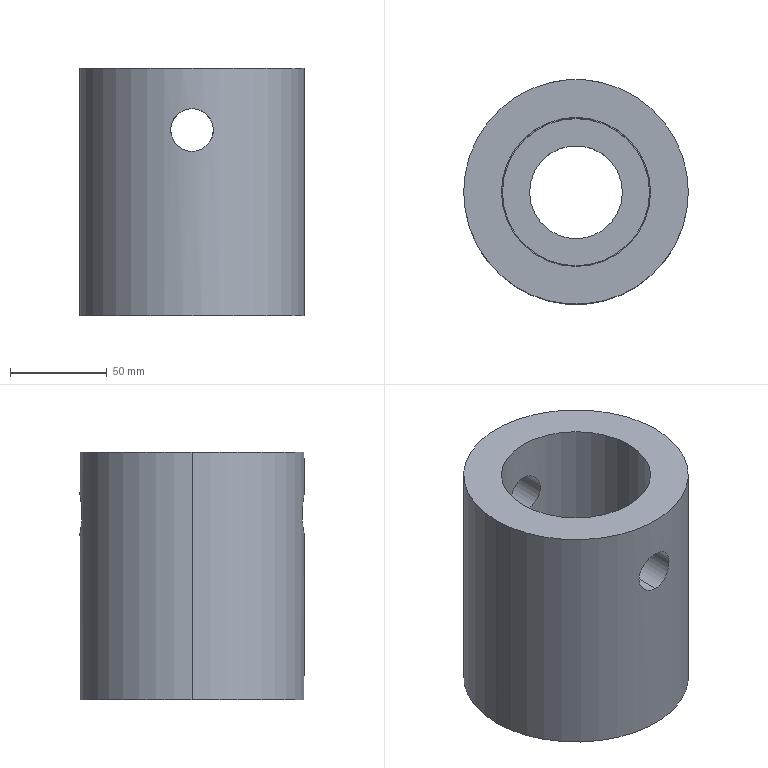Part | SolidWorks | features ICE 4, Extrusion 1 | 1 solid | 19 faces | box 116 x 116 x 128 mm | volume 818395 mm3 | cylinder 14 | plane 5 | commonest cylinder face diameters 22 x4 48 x2 76 x2 77 x2 80 x2 116 x2
STEP:
#1=CARTESIAN_POINT('',(-40.,0.,64.));
#2=VERTEX_POINT('',#1);
#3=CARTESIAN_POINT('',(40.,0.,64.));
#4=VERTEX_POINT('',#3);
#5=CARTESIAN_POINT('',(0.,0.,64.));
#6=DIRECTION('',(0.,0.,1.));
#7=DIRECTION('',(1.,0.,0.));
#8=AXIS2_PLACEMENT_3D('',#5,#6,#7);
#9=CIRCLE('',#8,40.);
#10=EDGE_CURVE('',#2,#4,#9,.T.);
#11=ORIENTED_EDGE('',*,*,#10,.T.);
#12=CARTESIAN_POINT('',(40.,0.,60.));
#13=VERTEX_POINT('',#12);
#14=CARTESIAN_POINT('',(40.,0.,64.));
#15=DIRECTION('',(0.,0.,-1.));
#16=VECTOR('',#15,1000.);
#17=LINE('',#14,#16);
#18=EDGE_CURVE('',#4,#13,#17,.T.);
#19=ORIENTED_EDGE('',*,*,#18,.T.);
#20=CARTESIAN_POINT('',(-40.,0.,60.));
#21=VERTEX_POINT('',#20);
#22=CARTESIAN_POINT('',(0.,0.,60.));
#23=DIRECTION('',(0.,0.,1.));
#24=DIRECTION('',(1.,0.,0.));
#25=AXIS2_PLACEMENT_3D('',#22,#23,#24);
#26=CIRCLE('',#25,40.);
#27=EDGE_CURVE('',#21,#13,#26,.T.);
#28=ORIENTED_EDGE('',*,*,#27,.F.);
#29=CARTESIAN_POINT('',(-40.,0.,64.));
#30=DIRECTION('',(0.,0.,-1.));
#31=VECTOR('',#30,1000.);
#32=LINE('',#29,#31);
#33=EDGE_CURVE('',#2,#21,#32,.T.);
#34=ORIENTED_EDGE('',*,*,#33,.F.);
#35=EDGE_LOOP('',(#11,#19,#28,#34));
#36=FACE_OUTER_BOUND('',#35,.T.);
#37=CARTESIAN_POINT('',(0.,0.,64.));
#38=DIRECTION('',(0.,0.,-1.));
#39=DIRECTION('',(-1.,0.,0.));
#40=AXIS2_PLACEMENT_3D('',#37,#38,#39);
#41=CYLINDRICAL_SURFACE('',#40,40.);
#42=ADVANCED_FACE('',(#36),#41,.F.);
#43=CARTESIAN_POINT('',(0.,-38.5,107.));
#44=VERTEX_POINT('',#43);
#45=CARTESIAN_POINT('',(0.,-38.5,85.));
#46=VERTEX_POINT('',#45);
#47=CARTESIAN_POINT('',(0.,-38.5,107.));
#48=CARTESIAN_POINT('',(0.7309,-38.5,107.));
#49=CARTESIAN_POINT('',(1.449,-38.479,106.928));
#50=CARTESIAN_POINT('',(2.507,-38.42,106.716));
#51=CARTESIAN_POINT('',(2.857,-38.395,106.629));
#52=CARTESIAN_POINT('',(3.55,-38.338,106.418));
#53=CARTESIAN_POINT('',(3.894,-38.304,106.294));
#54=CARTESIAN_POINT('',(4.892,-38.194,105.879));
#55=CARTESIAN_POINT('',(5.522,-38.107,105.541));
#56=CARTESIAN_POINT('',(6.417,-37.963,104.942));
#57=CARTESIAN_POINT('',(6.708,-37.912,104.725));
#58=CARTESIAN_POINT('',(7.264,-37.81,104.268));
#59=CARTESIAN_POINT('',(7.529,-37.758,104.028));
#60=CARTESIAN_POINT('',(8.285,-37.601,103.271));
#61=CARTESIAN_POINT('',(8.739,-37.497,102.719));
#62=CARTESIAN_POINT('',(9.543,-37.301,101.518));
#63=CARTESIAN_POINT('',(9.882,-37.211,100.884));
#64=CARTESIAN_POINT('',(10.294,-37.098,99.893));
#65=CARTESIAN_POINT('',(10.416,-37.064,99.555));
#66=CARTESIAN_POINT('',(10.627,-37.005,98.864));
#67=CARTESIAN_POINT('',(10.716,-36.979,98.509));
#68=CARTESIAN_POINT('',(10.929,-36.917,97.443));
#69=CARTESIAN_POINT('',(11.,-36.895,96.727));
#70=CARTESIAN_POINT('',(11.,-36.895,95.283));
#71=CARTESIAN_POINT('',(10.928,-36.917,94.55));
#72=CARTESIAN_POINT('',(10.645,-36.999,93.136));
#73=CARTESIAN_POINT('',(10.436,-37.06,92.448));
#74=CARTESIAN_POINT('',(10.019,-37.174,91.446));
#75=CARTESIAN_POINT('',(9.863,-37.215,91.117));
#76=CARTESIAN_POINT('',(9.524,-37.304,90.484));
#77=CARTESIAN_POINT('',(9.339,-37.351,90.177));
#78=CARTESIAN_POINT('',(8.942,-37.448,89.584));
#79=CARTESIAN_POINT('',(8.729,-37.498,89.297));
#80=CARTESIAN_POINT('',(8.274,-37.601,88.742));
#81=CARTESIAN_POINT('',(8.03,-37.654,88.474));
#82=CARTESIAN_POINT('',(7.267,-37.811,87.711));
#83=CARTESIAN_POINT('',(6.716,-37.914,87.259));
#84=CARTESIAN_POINT('',(5.527,-38.106,86.463));
#85=CARTESIAN_POINT('',(4.883,-38.195,86.117));
#86=CARTESIAN_POINT('',(3.556,-38.341,85.566));
#87=CARTESIAN_POINT('',(2.87,-38.399,85.356));
#88=CARTESIAN_POINT('',(1.805,-38.459,85.143));
#89=CARTESIAN_POINT('',(1.443,-38.475,85.089));
#90=CARTESIAN_POINT('',(0.7207,-38.495,85.018));
#91=CARTESIAN_POINT('',(0.3602,-38.5,85.));
#92=CARTESIAN_POINT('',(0.,-38.5,85.));
#93=B_SPLINE_CURVE_WITH_KNOTS('',3,(#47,#48,#49,#50,#51,#52,#53,#54,#55,#56,#57,#58,#59,#60,#61,#62,#63,#64,#65,#66,#67,#68,#69,#70,#71,#72,#73,#74,#75,#76,#77,#78,#79,#80,#81,#82,#83,#84,#85,#86,#87,#88,#89,#90,#91,#92),.UNSPECIFIED.,.F.,.F.,(4,2,2,2,2,2,2,2,2,2,2,2,2,2,2,2,2,2,2,2,2,2,4),(0.,0.002161,0.003241,0.004322,0.006482,0.007563,0.008643,0.0108,0.01296,0.01404,0.01513,0.01729,0.01945,0.02161,0.02269,0.02377,0.02485,0.02593,0.02809,0.03025,0.03241,0.03349,0.03457),.UNSPECIFIED.);
#94=EDGE_CURVE('',#44,#46,#93,.T.);
#95=ORIENTED_EDGE('',*,*,#94,.F.);
#96=CARTESIAN_POINT('',(0.,-38.5,85.));
#97=CARTESIAN_POINT('',(-0.3601,-38.5,85.));
#98=CARTESIAN_POINT('',(-0.7197,-38.495,85.018));
#99=CARTESIAN_POINT('',(-1.438,-38.475,85.088));
#100=CARTESIAN_POINT('',(-1.798,-38.46,85.142));
#101=CARTESIAN_POINT('',(-2.87,-38.4,85.356));
#102=CARTESIAN_POINT('',(-3.557,-38.341,85.566));
#103=CARTESIAN_POINT('',(-4.552,-38.231,85.979));
#104=CARTESIAN_POINT('',(-4.877,-38.191,86.133));
#105=CARTESIAN_POINT('',(-5.514,-38.104,86.475));
#106=CARTESIAN_POINT('',(-5.825,-38.058,86.662));
#107=CARTESIAN_POINT('',(-6.718,-37.914,87.26));
#108=CARTESIAN_POINT('',(-7.269,-37.811,87.713));
#109=CARTESIAN_POINT('',(-8.03,-37.654,88.474));
#110=CARTESIAN_POINT('',(-8.274,-37.601,88.743));
#111=CARTESIAN_POINT('',(-8.73,-37.498,89.298));
#112=CARTESIAN_POINT('',(-8.943,-37.448,89.585));
#113=CARTESIAN_POINT('',(-9.538,-37.302,90.474));
#114=CARTESIAN_POINT('',(-9.877,-37.212,91.105));
#115=CARTESIAN_POINT('',(-10.435,-37.06,92.446));
#116=CARTESIAN_POINT('',(-10.645,-37.,93.135));
#117=CARTESIAN_POINT('',(-10.856,-36.938,94.191));
#118=CARTESIAN_POINT('',(-10.91,-36.922,94.548));
#119=CARTESIAN_POINT('',(-10.982,-36.901,95.269));
#120=CARTESIAN_POINT('',(-11.,-36.895,95.636));
#121=CARTESIAN_POINT('',(-11.,-36.895,96.723));
#122=CARTESIAN_POINT('',(-10.929,-36.916,97.44));
#123=CARTESIAN_POINT('',(-10.718,-36.978,98.502));
#124=CARTESIAN_POINT('',(-10.629,-37.004,98.855));
#125=CARTESIAN_POINT('',(-10.418,-37.064,99.55));
#126=CARTESIAN_POINT('',(-10.296,-37.098,99.889));
#127=CARTESIAN_POINT('',(-9.883,-37.211,100.883));
#128=CARTESIAN_POINT('',(-9.545,-37.3,101.515));
#129=CARTESIAN_POINT('',(-8.741,-37.497,102.716));
#130=CARTESIAN_POINT('',(-8.286,-37.601,103.27));
#131=CARTESIAN_POINT('',(-7.53,-37.757,104.027));
#132=CARTESIAN_POINT('',(-7.265,-37.809,104.267));
#133=CARTESIAN_POINT('',(-6.711,-37.912,104.723));
#134=CARTESIAN_POINT('',(-6.419,-37.962,104.94));
#135=CARTESIAN_POINT('',(-5.523,-38.107,105.54));
#136=CARTESIAN_POINT('',(-4.893,-38.194,105.878));
#137=CARTESIAN_POINT('',(-3.568,-38.34,106.43));
#138=CARTESIAN_POINT('',(-2.866,-38.4,106.645));
#139=CARTESIAN_POINT('',(-1.45,-38.479,106.928));
#140=CARTESIAN_POINT('',(-0.7307,-38.5,107.));
#141=CARTESIAN_POINT('',(0.,-38.5,107.));
#142=B_SPLINE_CURVE_WITH_KNOTS('',3,(#96,#97,#98,#99,#100,#101,#102,#103,#104,#105,#106,#107,#108,#109,#110,#111,#112,#113,#114,#115,#116,#117,#118,#119,#120,#121,#122,#123,#124,#125,#126,#127,#128,#129,#130,#131,#132,#133,#134,#135,#136,#137,#138,#139,#140,#141),.UNSPECIFIED.,.F.,.F.,(4,2,2,2,2,2,2,2,2,2,2,2,2,2,2,2,2,2,2,2,2,2,4),(0.03457,0.03565,0.03673,0.03889,0.03997,0.04105,0.04321,0.04429,0.04537,0.04753,0.04969,0.05077,0.05185,0.05401,0.05509,0.05617,0.05833,0.06049,0.06157,0.06265,0.06481,0.06697,0.06913),.UNSPECIFIED.);
#143=EDGE_CURVE('',#46,#44,#142,.T.);
#144=ORIENTED_EDGE('',*,*,#143,.F.);
#145=EDGE_LOOP('',(#95,#144));
#146=FACE_BOUND('',#145,.T.);
#147=CARTESIAN_POINT('',(38.5,0.,64.));
#148=VERTEX_POINT('',#147);
#149=CARTESIAN_POINT('',(-38.5,0.,64.));
#150=VERTEX_POINT('',#149);
#151=CARTESIAN_POINT('',(0.,0.,64.));
#152=DIRECTION('',(0.,0.,-1.));
#153=DIRECTION('',(1.,0.,0.));
#154=AXIS2_PLACEMENT_3D('',#151,#152,#153);
#155=CIRCLE('',#154,38.5);
#156=EDGE_CURVE('',#148,#150,#155,.T.);
#157=ORIENTED_EDGE('',*,*,#156,.T.);
#158=CARTESIAN_POINT('',(-38.5,0.,128.));
#159=VERTEX_POINT('',#158);
#160=CARTESIAN_POINT('',(-38.5,0.,60.));
#161=DIRECTION('',(0.,0.,1.));
#162=VECTOR('',#161,1000.);
#163=LINE('',#160,#162);
#164=EDGE_CURVE('',#150,#159,#163,.T.);
#165=ORIENTED_EDGE('',*,*,#164,.T.);
#166=CARTESIAN_POINT('',(38.5,0.,128.));
#167=VERTEX_POINT('',#166);
#168=CARTESIAN_POINT('',(0.,0.,128.));
#169=DIRECTION('',(0.,0.,1.));
#170=DIRECTION('',(1.,0.,0.));
#171=AXIS2_PLACEMENT_3D('',#168,#169,#170);
#172=CIRCLE('',#171,38.5);
#173=EDGE_CURVE('',#159,#167,#172,.T.);
#174=ORIENTED_EDGE('',*,*,#173,.T.);
#175=CARTESIAN_POINT('',(38.5,0.,60.));
#176=DIRECTION('',(0.,0.,1.));
#177=VECTOR('',#176,1000.);
#178=LINE('',#175,#177);
#179=EDGE_CURVE('',#148,#167,#178,.T.);
#180=ORIENTED_EDGE('',*,*,#179,.F.);
#181=EDGE_LOOP('',(#157,#165,#174,#180));
#182=FACE_OUTER_BOUND('',#181,.T.);
#183=CARTESIAN_POINT('',(0.,0.,60.));
#184=DIRECTION('',(0.,0.,1.));
#185=DIRECTION('',(1.,0.,0.));
#186=AXIS2_PLACEMENT_3D('',#183,#184,#185);
#187=CYLINDRICAL_SURFACE('',#186,38.5);
#188=ADVANCED_FACE('',(#146,#182),#187,.F.);
#189=CARTESIAN_POINT('',(0.,-58.,85.));
#190=VERTEX_POINT('',#189);
#191=CARTESIAN_POINT('',(0.,-58.,107.));
#192=VERTEX_POINT('',#191);
#193=CARTESIAN_POINT('',(0.,-58.,85.));
#194=CARTESIAN_POINT('',(-0.7186,-58.,85.));
#195=CARTESIAN_POINT('',(-1.434,-57.987,85.07));
#196=CARTESIAN_POINT('',(-2.502,-57.947,85.282));
#197=CARTESIAN_POINT('',(-2.855,-57.931,85.371));
#198=CARTESIAN_POINT('',(-3.543,-57.893,85.58));
#199=CARTESIAN_POINT('',(-3.881,-57.871,85.701));
#200=CARTESIAN_POINT('',(-4.543,-57.823,85.975));
#201=CARTESIAN_POINT('',(-4.867,-57.796,86.129));
#202=CARTESIAN_POINT('',(-5.503,-57.739,86.469));
#203=CARTESIAN_POINT('',(-5.815,-57.709,86.656));
#204=CARTESIAN_POINT('',(-6.714,-57.613,87.257));
#205=CARTESIAN_POINT('',(-7.266,-57.545,87.711));
#206=CARTESIAN_POINT('',(-8.281,-57.408,88.724));
#207=CARTESIAN_POINT('',(-8.745,-57.338,89.289));
#208=CARTESIAN_POINT('',(-9.541,-57.211,90.48));
#209=CARTESIAN_POINT('',(-9.88,-57.153,91.11));
#210=CARTESIAN_POINT('',(-10.296,-57.079,92.111));
#211=CARTESIAN_POINT('',(-10.419,-57.057,92.454));
#212=CARTESIAN_POINT('',(-10.629,-57.018,93.144));
#213=CARTESIAN_POINT('',(-10.804,-56.985,93.841));
#214=CARTESIAN_POINT('',(-10.91,-56.965,94.551));
#215=CARTESIAN_POINT('',(-10.981,-56.951,95.268));
#216=CARTESIAN_POINT('',(-11.,-56.947,95.631));
#217=CARTESIAN_POINT('',(-11.,-56.947,96.721));
#218=CARTESIAN_POINT('',(-10.93,-56.961,97.436));
#219=CARTESIAN_POINT('',(-10.72,-57.001,98.493));
#220=CARTESIAN_POINT('',(-10.633,-57.017,98.842));
#221=CARTESIAN_POINT('',(-10.422,-57.056,99.536));
#222=CARTESIAN_POINT('',(-10.3,-57.078,99.878));
#223=CARTESIAN_POINT('',(-9.887,-57.152,100.875));
#224=CARTESIAN_POINT('',(-9.549,-57.21,101.507));
#225=CARTESIAN_POINT('',(-8.95,-57.306,102.405));
#226=CARTESIAN_POINT('',(-8.734,-57.339,102.697));
#227=CARTESIAN_POINT('',(-8.277,-57.407,103.254));
#228=CARTESIAN_POINT('',(-8.036,-57.441,103.52));
#229=CARTESIAN_POINT('',(-7.278,-57.544,104.279));
#230=CARTESIAN_POINT('',(-6.725,-57.612,104.735));
#231=CARTESIAN_POINT('',(-5.52,-57.74,105.542));
#232=CARTESIAN_POINT('',(-4.887,-57.798,105.881));
#233=CARTESIAN_POINT('',(-3.895,-57.87,106.293));
#234=CARTESIAN_POINT('',(-3.557,-57.892,106.415));
#235=CARTESIAN_POINT('',(-2.867,-57.93,106.626));
#236=CARTESIAN_POINT('',(-2.512,-57.947,106.715));
#237=CARTESIAN_POINT('',(-1.448,-57.986,106.928));
#238=CARTESIAN_POINT('',(-0.7284,-58.,107.));
#239=CARTESIAN_POINT('',(0.,-58.,107.));
#240=B_SPLINE_CURVE_WITH_KNOTS('',3,(#193,#194,#195,#196,#197,#198,#199,#200,#201,#202,#203,#204,#205,#206,#207,#208,#209,#210,#211,#212,#213,#214,#215,#216,#217,#218,#219,#220,#221,#222,#223,#224,#225,#226,#227,#228,#229,#230,#231,#232,#233,#234,#235,#236,#237,#238,#239),.UNSPECIFIED.,.F.,.F.,(4,2,2,2,2,2,2,2,2,2,1,2,2,2,2,2,2,2,2,2,2,2,2,4),(0.03447,0.03662,0.0377,0.03878,0.03985,0.04093,0.04308,0.04524,0.04739,0.04847,0.04955,0.05062,0.0517,0.05385,0.05493,0.05601,0.05816,0.05924,0.06031,0.06247,0.06462,0.0657,0.06678,0.06893),.UNSPECIFIED.);
#241=EDGE_CURVE('',#190,#192,#240,.T.);
#242=ORIENTED_EDGE('',*,*,#241,.F.);
#243=CARTESIAN_POINT('',(0.,-58.,85.));
#244=DIRECTION('',(0.,1.,0.));
#245=VECTOR('',#244,1000.);
#246=LINE('',#243,#245);
#247=EDGE_CURVE('',#190,#46,#246,.T.);
#248=ORIENTED_EDGE('',*,*,#247,.T.);
#249=ORIENTED_EDGE('',*,*,#143,.T.);
#250=CARTESIAN_POINT('',(0.,-58.,107.));
#251=DIRECTION('',(0.,1.,0.));
#252=VECTOR('',#251,1000.);
#253=LINE('',#250,#252);
#254=EDGE_CURVE('',#192,#44,#253,.T.);
#255=ORIENTED_EDGE('',*,*,#254,.F.);
#256=EDGE_LOOP('',(#242,#248,#249,#255));
#257=FACE_OUTER_BOUND('',#256,.T.);
#258=CARTESIAN_POINT('',(0.,-58.,96.));
#259=DIRECTION('',(0.,1.,0.));
#260=DIRECTION('',(0.,0.,1.));
#261=AXIS2_PLACEMENT_3D('',#258,#259,#260);
#262=CYLINDRICAL_SURFACE('',#261,11.);
#263=ADVANCED_FACE('',(#257),#262,.F.);
#264=CARTESIAN_POINT('',(0.,38.5,107.));
#265=VERTEX_POINT('',#264);
#266=CARTESIAN_POINT('',(0.,38.5,85.));
#267=VERTEX_POINT('',#266);
#268=CARTESIAN_POINT('',(0.,38.5,107.));
#269=CARTESIAN_POINT('',(-0.7309,38.5,107.));
#270=CARTESIAN_POINT('',(-1.449,38.479,106.928));
#271=CARTESIAN_POINT('',(-2.507,38.42,106.716));
#272=CARTESIAN_POINT('',(-2.857,38.395,106.629));
#273=CARTESIAN_POINT('',(-3.55,38.338,106.418));
#274=CARTESIAN_POINT('',(-3.894,38.304,106.294));
#275=CARTESIAN_POINT('',(-4.892,38.194,105.879));
#276=CARTESIAN_POINT('',(-5.522,38.107,105.541));
#277=CARTESIAN_POINT('',(-6.417,37.963,104.942));
#278=CARTESIAN_POINT('',(-6.708,37.912,104.725));
#279=CARTESIAN_POINT('',(-7.264,37.81,104.268));
#280=CARTESIAN_POINT('',(-7.529,37.758,104.028));
#281=CARTESIAN_POINT('',(-8.285,37.601,103.271));
#282=CARTESIAN_POINT('',(-8.739,37.497,102.719));
#283=CARTESIAN_POINT('',(-9.543,37.301,101.518));
#284=CARTESIAN_POINT('',(-9.882,37.211,100.884));
#285=CARTESIAN_POINT('',(-10.294,37.098,99.893));
#286=CARTESIAN_POINT('',(-10.416,37.064,99.555));
#287=CARTESIAN_POINT('',(-10.627,37.005,98.864));
#288=CARTESIAN_POINT('',(-10.716,36.979,98.509));
#289=CARTESIAN_POINT('',(-10.929,36.917,97.443));
#290=CARTESIAN_POINT('',(-11.,36.895,96.727));
#291=CARTESIAN_POINT('',(-11.,36.895,95.283));
#292=CARTESIAN_POINT('',(-10.928,36.917,94.55));
#293=CARTESIAN_POINT('',(-10.645,36.999,93.136));
#294=CARTESIAN_POINT('',(-10.436,37.06,92.448));
#295=CARTESIAN_POINT('',(-10.019,37.174,91.446));
#296=CARTESIAN_POINT('',(-9.863,37.215,91.117));
#297=CARTESIAN_POINT('',(-9.524,37.304,90.484));
#298=CARTESIAN_POINT('',(-9.339,37.351,90.177));
#299=CARTESIAN_POINT('',(-8.942,37.448,89.584));
#300=CARTESIAN_POINT('',(-8.729,37.498,89.297));
#301=CARTESIAN_POINT('',(-8.274,37.601,88.742));
#302=CARTESIAN_POINT('',(-8.03,37.654,88.474));
#303=CARTESIAN_POINT('',(-7.267,37.811,87.711));
#304=CARTESIAN_POINT('',(-6.716,37.914,87.259));
#305=CARTESIAN_POINT('',(-5.527,38.106,86.463));
#306=CARTESIAN_POINT('',(-4.883,38.195,86.117));
#307=CARTESIAN_POINT('',(-3.556,38.341,85.566));
#308=CARTESIAN_POINT('',(-2.87,38.399,85.356));
#309=CARTESIAN_POINT('',(-1.805,38.459,85.143));
#310=CARTESIAN_POINT('',(-1.443,38.475,85.089));
#311=CARTESIAN_POINT('',(-0.7207,38.495,85.018));
#312=CARTESIAN_POINT('',(-0.3602,38.5,85.));
#313=CARTESIAN_POINT('',(0.,38.5,85.));
#314=B_SPLINE_CURVE_WITH_KNOTS('',3,(#268,#269,#270,#271,#272,#273,#274,#275,#276,#277,#278,#279,#280,#281,#282,#283,#284,#285,#286,#287,#288,#289,#290,#291,#292,#293,#294,#295,#296,#297,#298,#299,#300,#301,#302,#303,#304,#305,#306,#307,#308,#309,#310,#311,#312,#313),.UNSPECIFIED.,.F.,.F.,(4,2,2,2,2,2,2,2,2,2,2,2,2,2,2,2,2,2,2,2,2,2,4),(0.,0.002161,0.003241,0.004322,0.006482,0.007563,0.008643,0.0108,0.01296,0.01404,0.01513,0.01729,0.01945,0.02161,0.02269,0.02377,0.02485,0.02593,0.02809,0.03025,0.03241,0.03349,0.03457),.UNSPECIFIED.);
#315=EDGE_CURVE('',#265,#267,#314,.T.);
#316=ORIENTED_EDGE('',*,*,#315,.T.);
#317=CARTESIAN_POINT('',(0.,58.,85.));
#318=VERTEX_POINT('',#317);
#319=CARTESIAN_POINT('',(0.,-58.,85.));
#320=DIRECTION('',(0.,1.,0.));
#321=VECTOR('',#320,1000.);
#322=LINE('',#319,#321);
#323=EDGE_CURVE('',#267,#318,#322,.T.);
#324=ORIENTED_EDGE('',*,*,#323,.T.);
#325=CARTESIAN_POINT('',(0.,58.,107.));
#326=VERTEX_POINT('',#325);
#327=CARTESIAN_POINT('',(0.,58.,107.));
#328=CARTESIAN_POINT('',(-0.7286,58.,107.));
#329=CARTESIAN_POINT('',(-1.445,57.986,106.928));
#330=CARTESIAN_POINT('',(-2.501,57.947,106.718));
#331=CARTESIAN_POINT('',(-2.85,57.931,106.631));
#332=CARTESIAN_POINT('',(-3.542,57.893,106.42));
#333=CARTESIAN_POINT('',(-3.885,57.871,106.297));
#334=CARTESIAN_POINT('',(-4.884,57.798,105.883));
#335=CARTESIAN_POINT('',(-5.515,57.74,105.545));
#336=CARTESIAN_POINT('',(-6.411,57.645,104.946));
#337=CARTESIAN_POINT('',(-6.703,57.612,104.73));
#338=CARTESIAN_POINT('',(-7.261,57.544,104.271));
#339=CARTESIAN_POINT('',(-7.527,57.51,104.029));
#340=CARTESIAN_POINT('',(-8.286,57.407,103.27));
#341=CARTESIAN_POINT('',(-8.741,57.339,102.717));
#342=CARTESIAN_POINT('',(-9.344,57.243,101.816));
#343=CARTESIAN_POINT('',(-9.531,57.212,101.504));
#344=CARTESIAN_POINT('',(-9.87,57.154,100.871));
#345=CARTESIAN_POINT('',(-10.023,57.128,100.547));
#346=CARTESIAN_POINT('',(-10.297,57.079,99.885));
#347=CARTESIAN_POINT('',(-10.419,57.057,99.547));
#348=CARTESIAN_POINT('',(-10.628,57.018,98.858));
#349=CARTESIAN_POINT('',(-10.717,57.001,98.504));
#350=CARTESIAN_POINT('',(-10.93,56.961,97.438));
#351=CARTESIAN_POINT('',(-11.,56.947,96.724));
#352=CARTESIAN_POINT('',(-11.,56.947,95.645));
#353=CARTESIAN_POINT('',(-10.983,56.951,95.284));
#354=CARTESIAN_POINT('',(-10.911,56.964,94.56));
#355=CARTESIAN_POINT('',(-10.858,56.975,94.201));
#356=CARTESIAN_POINT('',(-10.647,57.015,93.142));
#357=CARTESIAN_POINT('',(-10.438,57.054,92.456));
#358=CARTESIAN_POINT('',(-10.024,57.127,91.455));
#359=CARTESIAN_POINT('',(-9.868,57.155,91.126));
#360=CARTESIAN_POINT('',(-9.527,57.212,90.49));
#361=CARTESIAN_POINT('',(-9.343,57.243,90.183));
#362=CARTESIAN_POINT('',(-8.945,57.306,89.588));
#363=CARTESIAN_POINT('',(-8.732,57.339,89.3));
#364=CARTESIAN_POINT('',(-8.277,57.407,88.745));
#365=CARTESIAN_POINT('',(-8.034,57.442,88.477));
#366=CARTESIAN_POINT('',(-7.266,57.545,87.71));
#367=CARTESIAN_POINT('',(-6.712,57.613,87.256));
#368=CARTESIAN_POINT('',(-5.82,57.708,86.659));
#369=CARTESIAN_POINT('',(-5.512,57.738,86.474));
#370=CARTESIAN_POINT('',(-4.875,57.796,86.133));
#371=CARTESIAN_POINT('',(-4.546,57.823,85.977));
#372=CARTESIAN_POINT('',(-3.548,57.895,85.563));
#373=CARTESIAN_POINT('',(-2.862,57.934,85.355));
#374=CARTESIAN_POINT('',(-1.802,57.973,85.143));
#375=CARTESIAN_POINT('',(-1.442,57.983,85.089));
#376=CARTESIAN_POINT('',(-0.7196,57.997,85.018));
#377=CARTESIAN_POINT('',(-0.3594,58.,85.));
#378=CARTESIAN_POINT('',(0.,58.,85.));
#379=B_SPLINE_CURVE_WITH_KNOTS('',3,(#327,#328,#329,#330,#331,#332,#333,#334,#335,#336,#337,#338,#339,#340,#341,#342,#343,#344,#345,#346,#347,#348,#349,#350,#351,#352,#353,#354,#355,#356,#357,#358,#359,#360,#361,#362,#363,#364,#365,#366,#367,#368,#369,#370,#371,#372,#373,#374,#375,#376,#377,#378),.UNSPECIFIED.,.F.,.F.,(4,2,2,2,2,2,2,2,2,2,2,2,2,2,2,2,2,2,2,2,2,2,2,2,2,4),(0.,0.002154,0.003231,0.004309,0.006463,0.00754,0.008617,0.01077,0.01185,0.01293,0.014,0.01508,0.01723,0.01831,0.01939,0.02154,0.02262,0.0237,0.02477,0.02585,0.02801,0.02908,0.03016,0.03231,0.03339,0.03447),.UNSPECIFIED.);
#380=EDGE_CURVE('',#326,#318,#379,.T.);
#381=ORIENTED_EDGE('',*,*,#380,.F.);
#382=CARTESIAN_POINT('',(0.,-58.,107.));
#383=DIRECTION('',(0.,1.,0.));
#384=VECTOR('',#383,1000.);
#385=LINE('',#382,#384);
#386=EDGE_CURVE('',#265,#326,#385,.T.);
#387=ORIENTED_EDGE('',*,*,#386,.F.);
#388=EDGE_LOOP('',(#316,#324,#381,#387));
#389=FACE_OUTER_BOUND('',#388,.T.);
#390=CARTESIAN_POINT('',(0.,-58.,96.));
#391=DIRECTION('',(0.,1.,0.));
#392=DIRECTION('',(0.,0.,1.));
#393=AXIS2_PLACEMENT_3D('',#390,#391,#392);
#394=CYLINDRICAL_SURFACE('',#393,11.);
#395=ADVANCED_FACE('',(#389),#394,.F.);
#396=ORIENTED_EDGE('',*,*,#380,.T.);
#397=CARTESIAN_POINT('',(0.,58.,85.));
#398=CARTESIAN_POINT('',(0.7186,58.,85.));
#399=CARTESIAN_POINT('',(1.434,57.987,85.07));
#400=CARTESIAN_POINT('',(2.502,57.947,85.282));
#401=CARTESIAN_POINT('',(2.855,57.931,85.371));
#402=CARTESIAN_POINT('',(3.543,57.893,85.58));
#403=CARTESIAN_POINT('',(3.881,57.871,85.701));
#404=CARTESIAN_POINT('',(4.543,57.823,85.975));
#405=CARTESIAN_POINT('',(4.867,57.796,86.129));
#406=CARTESIAN_POINT('',(5.503,57.739,86.469));
#407=CARTESIAN_POINT('',(5.815,57.709,86.656));
#408=CARTESIAN_POINT('',(6.714,57.613,87.257));
#409=CARTESIAN_POINT('',(7.266,57.545,87.711));
#410=CARTESIAN_POINT('',(8.281,57.408,88.724));
#411=CARTESIAN_POINT('',(8.745,57.338,89.289));
#412=CARTESIAN_POINT('',(9.541,57.211,90.48));
#413=CARTESIAN_POINT('',(9.88,57.153,91.11));
#414=CARTESIAN_POINT('',(10.296,57.079,92.111));
#415=CARTESIAN_POINT('',(10.419,57.057,92.454));
#416=CARTESIAN_POINT('',(10.629,57.018,93.144));
#417=CARTESIAN_POINT('',(10.804,56.985,93.841));
#418=CARTESIAN_POINT('',(10.91,56.965,94.551));
#419=CARTESIAN_POINT('',(10.981,56.951,95.268));
#420=CARTESIAN_POINT('',(11.,56.947,95.631));
#421=CARTESIAN_POINT('',(11.,56.947,96.721));
#422=CARTESIAN_POINT('',(10.93,56.961,97.436));
#423=CARTESIAN_POINT('',(10.72,57.001,98.493));
#424=CARTESIAN_POINT('',(10.633,57.017,98.842));
#425=CARTESIAN_POINT('',(10.422,57.056,99.536));
#426=CARTESIAN_POINT('',(10.3,57.078,99.878));
#427=CARTESIAN_POINT('',(9.887,57.152,100.875));
#428=CARTESIAN_POINT('',(9.549,57.21,101.507));
#429=CARTESIAN_POINT('',(8.95,57.306,102.405));
#430=CARTESIAN_POINT('',(8.734,57.339,102.697));
#431=CARTESIAN_POINT('',(8.277,57.407,103.254));
#432=CARTESIAN_POINT('',(8.036,57.441,103.52));
#433=CARTESIAN_POINT('',(7.278,57.544,104.279));
#434=CARTESIAN_POINT('',(6.725,57.612,104.735));
#435=CARTESIAN_POINT('',(5.52,57.74,105.542));
#436=CARTESIAN_POINT('',(4.887,57.798,105.881));
#437=CARTESIAN_POINT('',(3.895,57.87,106.293));
#438=CARTESIAN_POINT('',(3.557,57.892,106.415));
#439=CARTESIAN_POINT('',(2.867,57.93,106.626));
#440=CARTESIAN_POINT('',(2.512,57.947,106.715));
#441=CARTESIAN_POINT('',(1.448,57.986,106.928));
#442=CARTESIAN_POINT('',(0.7284,58.,107.));
#443=CARTESIAN_POINT('',(0.,58.,107.));
#444=B_SPLINE_CURVE_WITH_KNOTS('',3,(#397,#398,#399,#400,#401,#402,#403,#404,#405,#406,#407,#408,#409,#410,#411,#412,#413,#414,#415,#416,#417,#418,#419,#420,#421,#422,#423,#424,#425,#426,#427,#428,#429,#430,#431,#432,#433,#434,#435,#436,#437,#438,#439,#440,#441,#442,#443),.UNSPECIFIED.,.F.,.F.,(4,2,2,2,2,2,2,2,2,2,1,2,2,2,2,2,2,2,2,2,2,2,2,4),(0.03447,0.03662,0.0377,0.03878,0.03985,0.04093,0.04308,0.04524,0.04739,0.04847,0.04955,0.05062,0.0517,0.05385,0.05493,0.05601,0.05816,0.05924,0.06031,0.06247,0.06462,0.0657,0.06678,0.06893),.UNSPECIFIED.);
#445=EDGE_CURVE('',#318,#326,#444,.T.);
#446=ORIENTED_EDGE('',*,*,#445,.T.);
#447=EDGE_LOOP('',(#396,#446));
#448=FACE_BOUND('',#447,.T.);
#449=CARTESIAN_POINT('',(58.,0.,128.));
#450=VERTEX_POINT('',#449);
#451=CARTESIAN_POINT('',(-58.,0.,128.));
#452=VERTEX_POINT('',#451);
#453=CARTESIAN_POINT('',(0.,0.,128.));
#454=DIRECTION('',(0.,0.,1.));
#455=DIRECTION('',(1.,0.,0.));
#456=AXIS2_PLACEMENT_3D('',#453,#454,#455);
#457=CIRCLE('',#456,58.);
#458=EDGE_CURVE('',#450,#452,#457,.T.);
#459=ORIENTED_EDGE('',*,*,#458,.F.);
#460=CARTESIAN_POINT('',(58.,0.,0.));
#461=VERTEX_POINT('',#460);
#462=CARTESIAN_POINT('',(58.,0.,128.));
#463=DIRECTION('',(0.,0.,-1.));
#464=VECTOR('',#463,1000.);
#465=LINE('',#462,#464);
#466=EDGE_CURVE('',#450,#461,#465,.T.);
#467=ORIENTED_EDGE('',*,*,#466,.T.);
#468=CARTESIAN_POINT('',(-58.,0.,0.));
#469=VERTEX_POINT('',#468);
#470=CARTESIAN_POINT('',(0.,0.,0.));
#471=DIRECTION('',(0.,0.,1.));
#472=DIRECTION('',(1.,0.,0.));
#473=AXIS2_PLACEMENT_3D('',#470,#471,#472);
#474=CIRCLE('',#473,58.);
#475=EDGE_CURVE('',#461,#469,#474,.T.);
#476=ORIENTED_EDGE('',*,*,#475,.T.);
#477=CARTESIAN_POINT('',(-58.,0.,128.));
#478=DIRECTION('',(0.,0.,-1.));
#479=VECTOR('',#478,1000.);
#480=LINE('',#477,#479);
#481=EDGE_CURVE('',#452,#469,#480,.T.);
#482=ORIENTED_EDGE('',*,*,#481,.F.);
#483=EDGE_LOOP('',(#459,#467,#476,#482));
#484=FACE_OUTER_BOUND('',#483,.T.);
#485=CARTESIAN_POINT('',(0.,0.,128.));
#486=DIRECTION('',(0.,0.,-1.));
#487=DIRECTION('',(-1.,0.,0.));
#488=AXIS2_PLACEMENT_3D('',#485,#486,#487);
#489=CYLINDRICAL_SURFACE('',#488,58.);
#490=ADVANCED_FACE('',(#448,#484),#489,.T.);
#491=CARTESIAN_POINT('',(-24.,0.,26.));
#492=VERTEX_POINT('',#491);
#493=CARTESIAN_POINT('',(24.,0.,26.));
#494=VERTEX_POINT('',#493);
#495=CARTESIAN_POINT('',(0.,0.,26.));
#496=DIRECTION('',(0.,0.,1.));
#497=DIRECTION('',(1.,0.,0.));
#498=AXIS2_PLACEMENT_3D('',#495,#496,#497);
#499=CIRCLE('',#498,24.);
#500=EDGE_CURVE('',#492,#494,#499,.T.);
#501=ORIENTED_EDGE('',*,*,#500,.T.);
#502=CARTESIAN_POINT('',(24.,0.,0.));
#503=VERTEX_POINT('',#502);
#504=CARTESIAN_POINT('',(24.,0.,128.));
#505=DIRECTION('',(0.,0.,-1.));
#506=VECTOR('',#505,1000.);
#507=LINE('',#504,#506);
#508=EDGE_CURVE('',#494,#503,#507,.T.);
#509=ORIENTED_EDGE('',*,*,#508,.T.);
#510=CARTESIAN_POINT('',(-24.,0.,0.));
#511=VERTEX_POINT('',#510);
#512=CARTESIAN_POINT('',(0.,0.,0.));
#513=DIRECTION('',(0.,0.,1.));
#514=DIRECTION('',(1.,0.,0.));
#515=AXIS2_PLACEMENT_3D('',#512,#513,#514);
#516=CIRCLE('',#515,24.);
#517=EDGE_CURVE('',#511,#503,#516,.T.);
#518=ORIENTED_EDGE('',*,*,#517,.F.);
#519=CARTESIAN_POINT('',(-24.,0.,128.));
#520=DIRECTION('',(0.,0.,-1.));
#521=VECTOR('',#520,1000.);
#522=LINE('',#519,#521);
#523=EDGE_CURVE('',#492,#511,#522,.T.);
#524=ORIENTED_EDGE('',*,*,#523,.F.);
#525=EDGE_LOOP('',(#501,#509,#518,#524));
#526=FACE_OUTER_BOUND('',#525,.T.);
#527=CARTESIAN_POINT('',(0.,0.,128.));
#528=DIRECTION('',(0.,0.,-1.));
#529=DIRECTION('',(-1.,0.,0.));
#530=AXIS2_PLACEMENT_3D('',#527,#528,#529);
#531=CYLINDRICAL_SURFACE('',#530,24.);
#532=ADVANCED_FACE('',(#526),#531,.F.);
#533=CARTESIAN_POINT('',(-38.,0.,26.));
#534=VERTEX_POINT('',#533);
#535=CARTESIAN_POINT('',(38.,0.,26.));
#536=VERTEX_POINT('',#535);
#537=CARTESIAN_POINT('',(0.,0.,26.));
#538=DIRECTION('',(0.,0.,1.));
#539=DIRECTION('',(1.,0.,0.));
#540=AXIS2_PLACEMENT_3D('',#537,#538,#539);
#541=CIRCLE('',#540,38.);
#542=EDGE_CURVE('',#534,#536,#541,.T.);
#543=ORIENTED_EDGE('',*,*,#542,.F.);
#544=CARTESIAN_POINT('',(-38.,0.,60.));
#545=VERTEX_POINT('',#544);
#546=CARTESIAN_POINT('',(-38.,0.,26.));
#547=DIRECTION('',(0.,0.,1.));
#548=VECTOR('',#547,1000.);
#549=LINE('',#546,#548);
#550=EDGE_CURVE('',#534,#545,#549,.T.);
#551=ORIENTED_EDGE('',*,*,#550,.T.);
#552=CARTESIAN_POINT('',(38.,0.,60.));
#553=VERTEX_POINT('',#552);
#554=CARTESIAN_POINT('',(0.,0.,60.));
#555=DIRECTION('',(0.,0.,-1.));
#556=DIRECTION('',(1.,0.,0.));
#557=AXIS2_PLACEMENT_3D('',#554,#555,#556);
#558=CIRCLE('',#557,38.);
#559=EDGE_CURVE('',#553,#545,#558,.T.);
#560=ORIENTED_EDGE('',*,*,#559,.F.);
#561=CARTESIAN_POINT('',(38.,0.,26.));
#562=DIRECTION('',(0.,0.,1.));
#563=VECTOR('',#562,1000.);
#564=LINE('',#561,#563);
#565=EDGE_CURVE('',#536,#553,#564,.T.);
#566=ORIENTED_EDGE('',*,*,#565,.F.);
#567=EDGE_LOOP('',(#543,#551,#560,#566));
#568=FACE_OUTER_BOUND('',#567,.T.);
#569=CARTESIAN_POINT('',(0.,0.,26.));
#570=DIRECTION('',(0.,0.,1.));
#571=DIRECTION('',(1.,0.,0.));
#572=AXIS2_PLACEMENT_3D('',#569,#570,#571);
#573=CYLINDRICAL_SURFACE('',#572,38.);
#574=ADVANCED_FACE('',(#568),#573,.F.);
#575=ORIENTED_EDGE('',*,*,#550,.F.);
#576=CARTESIAN_POINT('',(0.,0.,26.));
#577=DIRECTION('',(0.,0.,1.));
#578=DIRECTION('',(1.,0.,0.));
#579=AXIS2_PLACEMENT_3D('',#576,#577,#578);
#580=CIRCLE('',#579,38.);
#581=EDGE_CURVE('',#536,#534,#580,.T.);
#582=ORIENTED_EDGE('',*,*,#581,.F.);
#583=ORIENTED_EDGE('',*,*,#565,.T.);
#584=CARTESIAN_POINT('',(0.,0.,60.));
#585=DIRECTION('',(0.,0.,-1.));
#586=DIRECTION('',(1.,0.,0.));
#587=AXIS2_PLACEMENT_3D('',#584,#585,#586);
#588=CIRCLE('',#587,38.);
#589=EDGE_CURVE('',#545,#553,#588,.T.);
#590=ORIENTED_EDGE('',*,*,#589,.F.);
#591=EDGE_LOOP('',(#575,#582,#583,#590));
#592=FACE_OUTER_BOUND('',#591,.T.);
#593=CARTESIAN_POINT('',(0.,0.,26.));
#594=DIRECTION('',(0.,0.,1.));
#595=DIRECTION('',(1.,0.,0.));
#596=AXIS2_PLACEMENT_3D('',#593,#594,#595);
#597=CYLINDRICAL_SURFACE('',#596,38.);
#598=ADVANCED_FACE('',(#592),#597,.F.);
#599=ORIENTED_EDGE('',*,*,#508,.F.);
#600=CARTESIAN_POINT('',(0.,0.,26.));
#601=DIRECTION('',(0.,0.,1.));
#602=DIRECTION('',(1.,0.,0.));
#603=AXIS2_PLACEMENT_3D('',#600,#601,#602);
#604=CIRCLE('',#603,24.);
#605=EDGE_CURVE('',#494,#492,#604,.T.);
#606=ORIENTED_EDGE('',*,*,#605,.T.);
#607=ORIENTED_EDGE('',*,*,#523,.T.);
#608=CARTESIAN_POINT('',(0.,0.,0.));
#609=DIRECTION('',(0.,0.,1.));
#610=DIRECTION('',(1.,0.,0.));
#611=AXIS2_PLACEMENT_3D('',#608,#609,#610);
#612=CIRCLE('',#611,24.);
#613=EDGE_CURVE('',#503,#511,#612,.T.);
#614=ORIENTED_EDGE('',*,*,#613,.F.);
#615=EDGE_LOOP('',(#599,#606,#607,#614));
#616=FACE_OUTER_BOUND('',#615,.T.);
#617=CARTESIAN_POINT('',(0.,0.,128.));
#618=DIRECTION('',(0.,0.,-1.));
#619=DIRECTION('',(-1.,0.,0.));
#620=AXIS2_PLACEMENT_3D('',#617,#618,#619);
#621=CYLINDRICAL_SURFACE('',#620,24.);
#622=ADVANCED_FACE('',(#616),#621,.F.);
#623=CARTESIAN_POINT('',(0.,0.,128.));
#624=DIRECTION('',(0.,0.,1.));
#625=DIRECTION('',(1.,0.,0.));
#626=AXIS2_PLACEMENT_3D('',#623,#624,#625);
#627=CIRCLE('',#626,38.5);
#628=EDGE_CURVE('',#167,#159,#627,.T.);
#629=ORIENTED_EDGE('',*,*,#628,.F.);
#630=ORIENTED_EDGE('',*,*,#173,.F.);
#631=EDGE_LOOP('',(#629,#630));
#632=FACE_BOUND('',#631,.T.);
#633=CARTESIAN_POINT('',(0.,0.,128.));
#634=DIRECTION('',(0.,0.,1.));
#635=DIRECTION('',(1.,0.,0.));
#636=AXIS2_PLACEMENT_3D('',#633,#634,#635);
#637=CIRCLE('',#636,58.);
#638=EDGE_CURVE('',#452,#450,#637,.T.);
#639=ORIENTED_EDGE('',*,*,#638,.T.);
#640=ORIENTED_EDGE('',*,*,#458,.T.);
#641=EDGE_LOOP('',(#639,#640));
#642=FACE_OUTER_BOUND('',#641,.T.);
#643=CARTESIAN_POINT('',(0.,0.,128.));
#644=DIRECTION('',(0.,0.,1.));
#645=DIRECTION('',(1.,0.,0.));
#646=AXIS2_PLACEMENT_3D('',#643,#644,#645);
#647=PLANE('',#646);
#648=ADVANCED_FACE('',(#632,#642),#647,.T.);
#649=CARTESIAN_POINT('',(0.,0.,0.));
#650=DIRECTION('',(0.,0.,1.));
#651=DIRECTION('',(1.,0.,0.));
#652=AXIS2_PLACEMENT_3D('',#649,#650,#651);
#653=CIRCLE('',#652,58.);
#654=EDGE_CURVE('',#469,#461,#653,.T.);
#655=ORIENTED_EDGE('',*,*,#654,.F.);
#656=ORIENTED_EDGE('',*,*,#475,.F.);
#657=EDGE_LOOP('',(#655,#656));
#658=FACE_OUTER_BOUND('',#657,.T.);
#659=ORIENTED_EDGE('',*,*,#517,.T.);
#660=ORIENTED_EDGE('',*,*,#613,.T.);
#661=EDGE_LOOP('',(#659,#660));
#662=FACE_BOUND('',#661,.T.);
#663=CARTESIAN_POINT('',(0.,0.,0.));
#664=DIRECTION('',(0.,0.,1.));
#665=DIRECTION('',(1.,0.,0.));
#666=AXIS2_PLACEMENT_3D('',#663,#664,#665);
#667=PLANE('',#666);
#668=ADVANCED_FACE('',(#658,#662),#667,.F.);
#669=ORIENTED_EDGE('',*,*,#466,.F.);
#670=ORIENTED_EDGE('',*,*,#638,.F.);
#671=ORIENTED_EDGE('',*,*,#481,.T.);
#672=ORIENTED_EDGE('',*,*,#654,.T.);
#673=EDGE_LOOP('',(#669,#670,#671,#672));
#674=FACE_OUTER_BOUND('',#673,.T.);
#675=CARTESIAN_POINT('',(0.,-58.,107.));
#676=CARTESIAN_POINT('',(0.7286,-58.,107.));
#677=CARTESIAN_POINT('',(1.445,-57.986,106.928));
#678=CARTESIAN_POINT('',(2.501,-57.947,106.718));
#679=CARTESIAN_POINT('',(2.85,-57.931,106.631));
#680=CARTESIAN_POINT('',(3.542,-57.893,106.42));
#681=CARTESIAN_POINT('',(3.885,-57.871,106.297));
#682=CARTESIAN_POINT('',(4.884,-57.798,105.883));
#683=CARTESIAN_POINT('',(5.515,-57.74,105.545));
#684=CARTESIAN_POINT('',(6.411,-57.645,104.946));
#685=CARTESIAN_POINT('',(6.703,-57.612,104.73));
#686=CARTESIAN_POINT('',(7.261,-57.544,104.271));
#687=CARTESIAN_POINT('',(7.527,-57.51,104.029));
#688=CARTESIAN_POINT('',(8.286,-57.407,103.27));
#689=CARTESIAN_POINT('',(8.741,-57.339,102.717));
#690=CARTESIAN_POINT('',(9.344,-57.243,101.816));
#691=CARTESIAN_POINT('',(9.531,-57.212,101.504));
#692=CARTESIAN_POINT('',(9.87,-57.154,100.871));
#693=CARTESIAN_POINT('',(10.023,-57.128,100.547));
#694=CARTESIAN_POINT('',(10.297,-57.079,99.885));
#695=CARTESIAN_POINT('',(10.419,-57.057,99.547));
#696=CARTESIAN_POINT('',(10.628,-57.018,98.858));
#697=CARTESIAN_POINT('',(10.717,-57.001,98.504));
#698=CARTESIAN_POINT('',(10.93,-56.961,97.438));
#699=CARTESIAN_POINT('',(11.,-56.947,96.724));
#700=CARTESIAN_POINT('',(11.,-56.947,95.645));
#701=CARTESIAN_POINT('',(10.983,-56.951,95.284));
#702=CARTESIAN_POINT('',(10.911,-56.964,94.56));
#703=CARTESIAN_POINT('',(10.858,-56.975,94.201));
#704=CARTESIAN_POINT('',(10.647,-57.015,93.142));
#705=CARTESIAN_POINT('',(10.438,-57.054,92.456));
#706=CARTESIAN_POINT('',(10.024,-57.127,91.455));
#707=CARTESIAN_POINT('',(9.868,-57.155,91.126));
#708=CARTESIAN_POINT('',(9.527,-57.212,90.49));
#709=CARTESIAN_POINT('',(9.343,-57.243,90.183));
#710=CARTESIAN_POINT('',(8.945,-57.306,89.588));
#711=CARTESIAN_POINT('',(8.732,-57.339,89.3));
#712=CARTESIAN_POINT('',(8.277,-57.407,88.745));
#713=CARTESIAN_POINT('',(8.034,-57.442,88.477));
#714=CARTESIAN_POINT('',(7.266,-57.545,87.71));
#715=CARTESIAN_POINT('',(6.712,-57.613,87.256));
#716=CARTESIAN_POINT('',(5.82,-57.708,86.659));
#717=CARTESIAN_POINT('',(5.512,-57.738,86.474));
#718=CARTESIAN_POINT('',(4.875,-57.796,86.133));
#719=CARTESIAN_POINT('',(4.546,-57.823,85.977));
#720=CARTESIAN_POINT('',(3.548,-57.895,85.563));
#721=CARTESIAN_POINT('',(2.862,-57.934,85.355));
#722=CARTESIAN_POINT('',(1.802,-57.973,85.143));
#723=CARTESIAN_POINT('',(1.442,-57.983,85.089));
#724=CARTESIAN_POINT('',(0.7196,-57.997,85.018));
#725=CARTESIAN_POINT('',(0.3594,-58.,85.));
#726=CARTESIAN_POINT('',(0.,-58.,85.));
#727=B_SPLINE_CURVE_WITH_KNOTS('',3,(#675,#676,#677,#678,#679,#680,#681,#682,#683,#684,#685,#686,#687,#688,#689,#690,#691,#692,#693,#694,#695,#696,#697,#698,#699,#700,#701,#702,#703,#704,#705,#706,#707,#708,#709,#710,#711,#712,#713,#714,#715,#716,#717,#718,#719,#720,#721,#722,#723,#724,#725,#726),.UNSPECIFIED.,.F.,.F.,(4,2,2,2,2,2,2,2,2,2,2,2,2,2,2,2,2,2,2,2,2,2,2,2,2,4),(0.,0.002154,0.003231,0.004309,0.006463,0.00754,0.008617,0.01077,0.01185,0.01293,0.014,0.01508,0.01723,0.01831,0.01939,0.02154,0.02262,0.0237,0.02477,0.02585,0.02801,0.02908,0.03016,0.03231,0.03339,0.03447),.UNSPECIFIED.);
#728=EDGE_CURVE('',#192,#190,#727,.T.);
#729=ORIENTED_EDGE('',*,*,#728,.T.);
#730=ORIENTED_EDGE('',*,*,#241,.T.);
#731=EDGE_LOOP('',(#729,#730));
#732=FACE_BOUND('',#731,.T.);
#733=CARTESIAN_POINT('',(0.,0.,128.));
#734=DIRECTION('',(0.,0.,-1.));
#735=DIRECTION('',(-1.,0.,0.));
#736=AXIS2_PLACEMENT_3D('',#733,#734,#735);
#737=CYLINDRICAL_SURFACE('',#736,58.);
#738=ADVANCED_FACE('',(#674,#732),#737,.T.);
#739=ORIENTED_EDGE('',*,*,#500,.F.);
#740=ORIENTED_EDGE('',*,*,#605,.F.);
#741=EDGE_LOOP('',(#739,#740));
#742=FACE_BOUND('',#741,.T.);
#743=ORIENTED_EDGE('',*,*,#581,.T.);
#744=ORIENTED_EDGE('',*,*,#542,.T.);
#745=EDGE_LOOP('',(#743,#744));
#746=FACE_OUTER_BOUND('',#745,.T.);
#747=CARTESIAN_POINT('',(0.,0.,26.));
#748=DIRECTION('',(0.,0.,1.));
#749=DIRECTION('',(1.,0.,0.));
#750=AXIS2_PLACEMENT_3D('',#747,#748,#749);
#751=PLANE('',#750);
#752=ADVANCED_FACE('',(#742,#746),#751,.T.);
#753=ORIENTED_EDGE('',*,*,#323,.F.);
#754=CARTESIAN_POINT('',(0.,38.5,85.));
#755=CARTESIAN_POINT('',(0.3601,38.5,85.));
#756=CARTESIAN_POINT('',(0.7197,38.495,85.018));
#757=CARTESIAN_POINT('',(1.438,38.475,85.088));
#758=CARTESIAN_POINT('',(1.798,38.46,85.142));
#759=CARTESIAN_POINT('',(2.87,38.4,85.356));
#760=CARTESIAN_POINT('',(3.557,38.341,85.566));
#761=CARTESIAN_POINT('',(4.552,38.231,85.979));
#762=CARTESIAN_POINT('',(4.877,38.191,86.133));
#763=CARTESIAN_POINT('',(5.514,38.104,86.475));
#764=CARTESIAN_POINT('',(5.825,38.058,86.662));
#765=CARTESIAN_POINT('',(6.718,37.914,87.26));
#766=CARTESIAN_POINT('',(7.269,37.811,87.713));
#767=CARTESIAN_POINT('',(8.03,37.654,88.474));
#768=CARTESIAN_POINT('',(8.274,37.601,88.743));
#769=CARTESIAN_POINT('',(8.73,37.498,89.298));
#770=CARTESIAN_POINT('',(8.943,37.448,89.585));
#771=CARTESIAN_POINT('',(9.538,37.302,90.474));
#772=CARTESIAN_POINT('',(9.877,37.212,91.105));
#773=CARTESIAN_POINT('',(10.435,37.06,92.446));
#774=CARTESIAN_POINT('',(10.645,37.,93.135));
#775=CARTESIAN_POINT('',(10.856,36.938,94.191));
#776=CARTESIAN_POINT('',(10.91,36.922,94.548));
#777=CARTESIAN_POINT('',(10.982,36.901,95.269));
#778=CARTESIAN_POINT('',(11.,36.895,95.636));
#779=CARTESIAN_POINT('',(11.,36.895,96.723));
#780=CARTESIAN_POINT('',(10.929,36.916,97.44));
#781=CARTESIAN_POINT('',(10.718,36.978,98.502));
#782=CARTESIAN_POINT('',(10.629,37.004,98.855));
#783=CARTESIAN_POINT('',(10.418,37.064,99.55));
#784=CARTESIAN_POINT('',(10.296,37.098,99.889));
#785=CARTESIAN_POINT('',(9.883,37.211,100.883));
#786=CARTESIAN_POINT('',(9.545,37.3,101.515));
#787=CARTESIAN_POINT('',(8.741,37.497,102.716));
#788=CARTESIAN_POINT('',(8.286,37.601,103.27));
#789=CARTESIAN_POINT('',(7.53,37.757,104.027));
#790=CARTESIAN_POINT('',(7.265,37.809,104.267));
#791=CARTESIAN_POINT('',(6.711,37.912,104.723));
#792=CARTESIAN_POINT('',(6.419,37.962,104.94));
#793=CARTESIAN_POINT('',(5.523,38.107,105.54));
#794=CARTESIAN_POINT('',(4.893,38.194,105.878));
#795=CARTESIAN_POINT('',(3.568,38.34,106.43));
#796=CARTESIAN_POINT('',(2.866,38.4,106.645));
#797=CARTESIAN_POINT('',(1.45,38.479,106.928));
#798=CARTESIAN_POINT('',(0.7307,38.5,107.));
#799=CARTESIAN_POINT('',(0.,38.5,107.));
#800=B_SPLINE_CURVE_WITH_KNOTS('',3,(#754,#755,#756,#757,#758,#759,#760,#761,#762,#763,#764,#765,#766,#767,#768,#769,#770,#771,#772,#773,#774,#775,#776,#777,#778,#779,#780,#781,#782,#783,#784,#785,#786,#787,#788,#789,#790,#791,#792,#793,#794,#795,#796,#797,#798,#799),.UNSPECIFIED.,.F.,.F.,(4,2,2,2,2,2,2,2,2,2,2,2,2,2,2,2,2,2,2,2,2,2,4),(0.03457,0.03565,0.03673,0.03889,0.03997,0.04105,0.04321,0.04429,0.04537,0.04753,0.04969,0.05077,0.05185,0.05401,0.05509,0.05617,0.05833,0.06049,0.06157,0.06265,0.06481,0.06697,0.06913),.UNSPECIFIED.);
#801=EDGE_CURVE('',#267,#265,#800,.T.);
#802=ORIENTED_EDGE('',*,*,#801,.T.);
#803=ORIENTED_EDGE('',*,*,#386,.T.);
#804=ORIENTED_EDGE('',*,*,#445,.F.);
#805=EDGE_LOOP('',(#753,#802,#803,#804));
#806=FACE_OUTER_BOUND('',#805,.T.);
#807=CARTESIAN_POINT('',(0.,-58.,96.));
#808=DIRECTION('',(0.,1.,0.));
#809=DIRECTION('',(0.,0.,1.));
#810=AXIS2_PLACEMENT_3D('',#807,#808,#809);
#811=CYLINDRICAL_SURFACE('',#810,11.);
#812=ADVANCED_FACE('',(#806),#811,.F.);
#813=ORIENTED_EDGE('',*,*,#247,.F.);
#814=ORIENTED_EDGE('',*,*,#728,.F.);
#815=ORIENTED_EDGE('',*,*,#254,.T.);
#816=ORIENTED_EDGE('',*,*,#94,.T.);
#817=EDGE_LOOP('',(#813,#814,#815,#816));
#818=FACE_OUTER_BOUND('',#817,.T.);
#819=CARTESIAN_POINT('',(0.,-58.,96.));
#820=DIRECTION('',(0.,1.,0.));
#821=DIRECTION('',(0.,0.,1.));
#822=AXIS2_PLACEMENT_3D('',#819,#820,#821);
#823=CYLINDRICAL_SURFACE('',#822,11.);
#824=ADVANCED_FACE('',(#818),#823,.F.);
#825=ORIENTED_EDGE('',*,*,#559,.T.);
#826=ORIENTED_EDGE('',*,*,#589,.T.);
#827=EDGE_LOOP('',(#825,#826));
#828=FACE_BOUND('',#827,.T.);
#829=ORIENTED_EDGE('',*,*,#27,.T.);
#830=CARTESIAN_POINT('',(0.,0.,60.));
#831=DIRECTION('',(0.,0.,1.));
#832=DIRECTION('',(1.,0.,0.));
#833=AXIS2_PLACEMENT_3D('',#830,#831,#832);
#834=CIRCLE('',#833,40.);
#835=EDGE_CURVE('',#13,#21,#834,.T.);
#836=ORIENTED_EDGE('',*,*,#835,.T.);
#837=EDGE_LOOP('',(#829,#836));
#838=FACE_OUTER_BOUND('',#837,.T.);
#839=CARTESIAN_POINT('',(0.,0.,60.));
#840=DIRECTION('',(0.,0.,1.));
#841=DIRECTION('',(1.,0.,0.));
#842=AXIS2_PLACEMENT_3D('',#839,#840,#841);
#843=PLANE('',#842);
#844=ADVANCED_FACE('',(#828,#838),#843,.T.);
#845=ORIENTED_EDGE('',*,*,#164,.F.);
#846=CARTESIAN_POINT('',(0.,0.,64.));
#847=DIRECTION('',(0.,0.,-1.));
#848=DIRECTION('',(1.,0.,0.));
#849=AXIS2_PLACEMENT_3D('',#846,#847,#848);
#850=CIRCLE('',#849,38.5);
#851=EDGE_CURVE('',#150,#148,#850,.T.);
#852=ORIENTED_EDGE('',*,*,#851,.T.);
#853=ORIENTED_EDGE('',*,*,#179,.T.);
#854=ORIENTED_EDGE('',*,*,#628,.T.);
#855=EDGE_LOOP('',(#845,#852,#853,#854));
#856=FACE_OUTER_BOUND('',#855,.T.);
#857=ORIENTED_EDGE('',*,*,#315,.F.);
#858=ORIENTED_EDGE('',*,*,#801,.F.);
#859=EDGE_LOOP('',(#857,#858));
#860=FACE_BOUND('',#859,.T.);
#861=CARTESIAN_POINT('',(0.,0.,60.));
#862=DIRECTION('',(0.,0.,1.));
#863=DIRECTION('',(1.,0.,0.));
#864=AXIS2_PLACEMENT_3D('',#861,#862,#863);
#865=CYLINDRICAL_SURFACE('',#864,38.5);
#866=ADVANCED_FACE('',(#856,#860),#865,.F.);
#867=ORIENTED_EDGE('',*,*,#10,.F.);
#868=CARTESIAN_POINT('',(0.,0.,64.));
#869=DIRECTION('',(0.,0.,1.));
#870=DIRECTION('',(1.,0.,0.));
#871=AXIS2_PLACEMENT_3D('',#868,#869,#870);
#872=CIRCLE('',#871,40.);
#873=EDGE_CURVE('',#4,#2,#872,.T.);
#874=ORIENTED_EDGE('',*,*,#873,.F.);
#875=EDGE_LOOP('',(#867,#874));
#876=FACE_OUTER_BOUND('',#875,.T.);
#877=ORIENTED_EDGE('',*,*,#156,.F.);
#878=ORIENTED_EDGE('',*,*,#851,.F.);
#879=EDGE_LOOP('',(#877,#878));
#880=FACE_BOUND('',#879,.T.);
#881=CARTESIAN_POINT('',(0.,0.,64.));
#882=DIRECTION('',(0.,0.,1.));
#883=DIRECTION('',(1.,0.,0.));
#884=AXIS2_PLACEMENT_3D('',#881,#882,#883);
#885=PLANE('',#884);
#886=ADVANCED_FACE('',(#876,#880),#885,.F.);
#887=ORIENTED_EDGE('',*,*,#18,.F.);
#888=ORIENTED_EDGE('',*,*,#873,.T.);
#889=ORIENTED_EDGE('',*,*,#33,.T.);
#890=ORIENTED_EDGE('',*,*,#835,.F.);
#891=EDGE_LOOP('',(#887,#888,#889,#890));
#892=FACE_OUTER_BOUND('',#891,.T.);
#893=CARTESIAN_POINT('',(0.,0.,64.));
#894=DIRECTION('',(0.,0.,-1.));
#895=DIRECTION('',(-1.,0.,0.));
#896=AXIS2_PLACEMENT_3D('',#893,#894,#895);
#897=CYLINDRICAL_SURFACE('',#896,40.);
#898=ADVANCED_FACE('',(#892),#897,.F.);
#899=CLOSED_SHELL('',(#42,#188,#263,#395,#490,#532,#574,#598,#622,#648,#668,#738,#752,#812,#824,#844,#866,#886,#898));
#900=MANIFOLD_SOLID_BREP('',#899);
#901=CARTESIAN_POINT('',(0.,0.,0.));
#902=DIRECTION('',(0.,0.,1.));
#903=DIRECTION('',(1.,0.,0.));
#904=AXIS2_PLACEMENT_3D('',#901,#902,#903);
#905=(LENGTH_UNIT()NAMED_UNIT(*)SI_UNIT(.MILLI.,.METRE.));
#906=UNCERTAINTY_MEASURE_WITH_UNIT(LENGTH_MEASURE(0.00001),#905,'','');
#907=(NAMED_UNIT(*)PLANE_ANGLE_UNIT()SI_UNIT($,.RADIAN.));
#908=(NAMED_UNIT(*)SI_UNIT($,.STERADIAN.)SOLID_ANGLE_UNIT());
#909=(GEOMETRIC_REPRESENTATION_CONTEXT(3)GLOBAL_UNCERTAINTY_ASSIGNED_CONTEXT((#906))GLOBAL_UNIT_ASSIGNED_CONTEXT((#905,#907,#908))REPRESENTATION_CONTEXT('',''));
#910=ADVANCED_BREP_SHAPE_REPRESENTATION('',(#900,#904),#909);